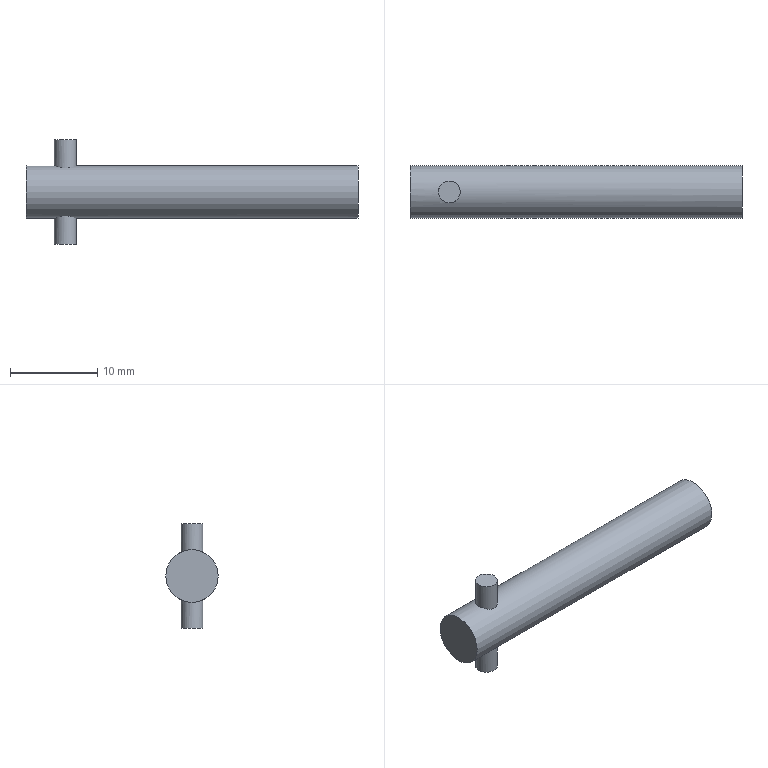Part | STEP file | 2-09.3 | 1 solid | 7 faces | box 38 x 6 x 12 mm | volume 1105 mm3 | plane 4 | cylinder 3 | commonest cylinder face diameters 2.5 x2 6 x1
STEP:
#1=CARTESIAN_POINT('',(0.,0.,0.));
#2=DIRECTION('',(0.,0.,1.));
#3=DIRECTION('',(1.,0.,0.));
#4=AXIS2_PLACEMENT_3D('',#1,#2,#3);
#5=CARTESIAN_POINT('',(0.,3.,0.));
#6=VERTEX_POINT('',#5);
#7=CARTESIAN_POINT('',(0.,0.,0.));
#8=DIRECTION('',(1.,0.,0.));
#9=DIRECTION('',(0.,1.,0.));
#10=AXIS2_PLACEMENT_3D('',#7,#8,#9);
#11=CIRCLE('',#10,3.);
#12=CARTESIAN_POINT('',(0.,-0.8038,0.));
#13=DIRECTION('',(1.,0.,0.));
#14=DIRECTION('',(0.,1.,0.));
#15=AXIS2_PLACEMENT_3D('',#12,#13,#14);
#16=PLANE('',#15);
#17=CARTESIAN_POINT('',(0.8038,0.));
#18=DIRECTION('',(1.,0.));
#19=AXIS2_PLACEMENT_2D('',#17,#18);
#20=CIRCLE('',#19,3.);
#21=(GEOMETRIC_REPRESENTATION_CONTEXT(2)PARAMETRIC_REPRESENTATION_CONTEXT()REPRESENTATION_CONTEXT('',''));
#22=DEFINITIONAL_REPRESENTATION('',(#20),#21);
#23=PCURVE('',#16,#22);
#24=CARTESIAN_POINT('',(0.,0.,0.));
#25=DIRECTION('',(1.,0.,0.));
#26=DIRECTION('',(0.,1.,0.));
#27=AXIS2_PLACEMENT_3D('',#24,#25,#26);
#28=CYLINDRICAL_SURFACE('',#27,3.);
#29=CARTESIAN_POINT('',(0.,0.));
#30=DIRECTION('',(1.,0.));
#31=VECTOR('',#30,1.);
#32=LINE('',#29,#31);
#33=(GEOMETRIC_REPRESENTATION_CONTEXT(2)PARAMETRIC_REPRESENTATION_CONTEXT()REPRESENTATION_CONTEXT('',''));
#34=DEFINITIONAL_REPRESENTATION('',(#32),#33);
#35=PCURVE('',#28,#34);
#36=SURFACE_CURVE('',#11,(#23,#35),.PCURVE_S1.);
#37=EDGE_CURVE('',#6,#6,#36,.T.);
#38=ORIENTED_EDGE('',*,*,#37,.T.);
#39=EDGE_LOOP('',(#38));
#40=FACE_BOUND('',#39,.F.);
#41=ADVANCED_FACE('',(#40),#16,.F.);
#42=CARTESIAN_POINT('',(38.,3.,0.));
#43=VERTEX_POINT('',#42);
#44=CARTESIAN_POINT('',(38.,0.,0.));
#45=DIRECTION('',(1.,0.,0.));
#46=DIRECTION('',(0.,1.,0.));
#47=AXIS2_PLACEMENT_3D('',#44,#45,#46);
#48=CIRCLE('',#47,3.);
#49=CARTESIAN_POINT('',(38.,-0.8038,0.));
#50=DIRECTION('',(1.,0.,0.));
#51=DIRECTION('',(0.,1.,0.));
#52=AXIS2_PLACEMENT_3D('',#49,#50,#51);
#53=PLANE('',#52);
#54=CARTESIAN_POINT('',(0.8038,0.));
#55=DIRECTION('',(1.,0.));
#56=AXIS2_PLACEMENT_2D('',#54,#55);
#57=CIRCLE('',#56,3.);
#58=(GEOMETRIC_REPRESENTATION_CONTEXT(2)PARAMETRIC_REPRESENTATION_CONTEXT()REPRESENTATION_CONTEXT('',''));
#59=DEFINITIONAL_REPRESENTATION('',(#57),#58);
#60=PCURVE('',#53,#59);
#61=CARTESIAN_POINT('',(0.,38.));
#62=DIRECTION('',(1.,0.));
#63=VECTOR('',#62,1.);
#64=LINE('',#61,#63);
#65=(GEOMETRIC_REPRESENTATION_CONTEXT(2)PARAMETRIC_REPRESENTATION_CONTEXT()REPRESENTATION_CONTEXT('',''));
#66=DEFINITIONAL_REPRESENTATION('',(#64),#65);
#67=PCURVE('',#28,#66);
#68=SURFACE_CURVE('',#48,(#60,#67),.PCURVE_S1.);
#69=EDGE_CURVE('',#43,#43,#68,.T.);
#70=ORIENTED_EDGE('',*,*,#69,.T.);
#71=EDGE_LOOP('',(#70));
#72=FACE_BOUND('',#71,.T.);
#73=ADVANCED_FACE('',(#72),#53,.T.);
#74=ORIENTED_EDGE('',*,*,#37,.T.);
#75=CARTESIAN_POINT('',(0.,3.,0.));
#76=DIRECTION('',(1.,0.,0.));
#77=VECTOR('',#76,1.);
#78=LINE('',#75,#77);
#79=CARTESIAN_POINT('',(6.283,0.));
#80=DIRECTION('',(0.,1.));
#81=VECTOR('',#80,1.);
#82=LINE('',#79,#81);
#83=(GEOMETRIC_REPRESENTATION_CONTEXT(2)PARAMETRIC_REPRESENTATION_CONTEXT()REPRESENTATION_CONTEXT('',''));
#84=DEFINITIONAL_REPRESENTATION('',(#82),#83);
#85=PCURVE('',#28,#84);
#86=CARTESIAN_POINT('',(0.,0.));
#87=DIRECTION('',(0.,1.));
#88=VECTOR('',#87,1.);
#89=LINE('',#86,#88);
#90=(GEOMETRIC_REPRESENTATION_CONTEXT(2)PARAMETRIC_REPRESENTATION_CONTEXT()REPRESENTATION_CONTEXT('',''));
#91=DEFINITIONAL_REPRESENTATION('',(#89),#90);
#92=PCURVE('',#28,#91);
#93=SEAM_CURVE('',#78,(#85,#92),.PCURVE_S1.);
#94=EDGE_CURVE('',#6,#43,#93,.T.);
#95=ORIENTED_EDGE('',*,*,#94,.T.);
#96=ORIENTED_EDGE('',*,*,#69,.F.);
#97=ORIENTED_EDGE('',*,*,#94,.F.);
#98=EDGE_LOOP('',(#74,#95,#96,#97));
#99=FACE_BOUND('',#98,.T.);
#100=CARTESIAN_POINT('',(3.25,0.,-3.));
#101=VERTEX_POINT('',#100);
#102=CARTESIAN_POINT('',(3.25,0.,-3.));
#103=CARTESIAN_POINT('',(3.25,0.187,-3.));
#104=CARTESIAN_POINT('',(3.376,0.7482,-2.948));
#105=CARTESIAN_POINT('',(3.851,1.128,-2.782));
#106=CARTESIAN_POINT('',(4.657,1.326,-2.694));
#107=CARTESIAN_POINT('',(5.12,1.178,-2.782));
#108=CARTESIAN_POINT('',(5.735,0.4976,-2.98));
#109=CARTESIAN_POINT('',(5.831,0.02602,-3.032));
#110=CARTESIAN_POINT('',(5.509,-0.9079,-2.903));
#111=CARTESIAN_POINT('',(5.038,-1.25,-2.727));
#112=CARTESIAN_POINT('',(3.853,-1.25,-2.727));
#113=CARTESIAN_POINT('',(3.315,-0.7572,-2.973));
#114=CARTESIAN_POINT('',(3.253,-0.08984,-2.999));
#115=CARTESIAN_POINT('',(3.251,-0.05135,-3.));
#116=CARTESIAN_POINT('',(3.25,-0.01284,-3.));
#117=CARTESIAN_POINT('',(3.25,0.,-3.));
#118=B_SPLINE_CURVE_WITH_KNOTS('',3,(#102,#103,#104,#105,#106,#107,#108,#109,#110,#111,#112,#113,#114,#115,#116,#117),.UNSPECIFIED.,.T.,.F.,(1,3,1,2,2,2,2,2,1,3,1),(-0.02386,0.,0.3333,1.,1.865,2.731,3.728,4.927,4.975,4.999,5.332),.UNSPECIFIED.);
#119=CARTESIAN_POINT('',(4.712,3.25));
#120=CARTESIAN_POINT('',(4.734,3.25));
#121=CARTESIAN_POINT('',(4.776,3.26));
#122=CARTESIAN_POINT('',(4.839,3.303));
#123=CARTESIAN_POINT('',(4.898,3.374));
#124=CARTESIAN_POINT('',(4.954,3.472));
#125=CARTESIAN_POINT('',(5.004,3.593));
#126=CARTESIAN_POINT('',(5.048,3.733));
#127=CARTESIAN_POINT('',(5.085,3.89));
#128=CARTESIAN_POINT('',(5.114,4.059));
#129=CARTESIAN_POINT('',(5.134,4.237));
#130=CARTESIAN_POINT('',(5.143,4.417));
#131=CARTESIAN_POINT('',(5.142,4.595));
#132=CARTESIAN_POINT('',(5.133,4.768));
#133=CARTESIAN_POINT('',(5.115,4.936));
#134=CARTESIAN_POINT('',(5.089,5.095));
#135=CARTESIAN_POINT('',(5.056,5.243));
#136=CARTESIAN_POINT('',(5.015,5.378));
#137=CARTESIAN_POINT('',(4.968,5.498));
#138=CARTESIAN_POINT('',(4.918,5.595));
#139=CARTESIAN_POINT('',(4.864,5.67));
#140=CARTESIAN_POINT('',(4.809,5.722));
#141=CARTESIAN_POINT('',(4.752,5.75));
#142=CARTESIAN_POINT('',(4.694,5.754));
#143=CARTESIAN_POINT('',(4.636,5.733));
#144=CARTESIAN_POINT('',(4.578,5.688));
#145=CARTESIAN_POINT('',(4.522,5.618));
#146=CARTESIAN_POINT('',(4.47,5.527));
#147=CARTESIAN_POINT('',(4.423,5.417));
#148=CARTESIAN_POINT('',(4.382,5.289));
#149=CARTESIAN_POINT('',(4.346,5.147));
#150=CARTESIAN_POINT('',(4.318,4.991));
#151=CARTESIAN_POINT('',(4.297,4.825));
#152=CARTESIAN_POINT('',(4.284,4.65));
#153=CARTESIAN_POINT('',(4.281,4.466));
#154=CARTESIAN_POINT('',(4.288,4.285));
#155=CARTESIAN_POINT('',(4.303,4.114));
#156=CARTESIAN_POINT('',(4.327,3.952));
#157=CARTESIAN_POINT('',(4.358,3.803));
#158=CARTESIAN_POINT('',(4.395,3.667));
#159=CARTESIAN_POINT('',(4.437,3.546));
#160=CARTESIAN_POINT('',(4.485,3.443));
#161=CARTESIAN_POINT('',(4.537,3.36));
#162=CARTESIAN_POINT('',(4.593,3.298));
#163=CARTESIAN_POINT('',(4.651,3.259));
#164=CARTESIAN_POINT('',(4.692,3.25));
#165=CARTESIAN_POINT('',(4.712,3.25));
#166=B_SPLINE_CURVE_WITH_KNOTS('',3,(#119,#120,#121,#122,#123,#124,#125,#126,#127,#128,#129,#130,#131,#132,#133,#134,#135,#136,#137,#138,#139,#140,#141,#142,#143,#144,#145,#146,#147,#148,#149,#150,#151,#152,#153,#154,#155,#156,#157,#158,#159,#160,#161,#162,#163,#164,#165),.UNSPECIFIED.,.T.,.F.,(4,1,1,1,1,1,1,1,1,1,1,1,1,1,1,1,1,1,1,1,1,1,1,1,1,1,1,1,1,1,1,1,1,1,1,1,1,1,1,1,1,1,1,1,4),(0.,0.1136,0.2272,0.3408,0.4544,0.568,0.6817,0.7953,0.9089,1.022,1.136,1.25,1.363,1.477,1.591,1.704,1.818,1.931,2.045,2.159,2.272,2.386,2.499,2.613,2.727,2.84,2.954,3.067,3.181,3.295,3.408,3.522,3.635,3.749,3.863,3.976,4.09,4.204,4.317,4.431,4.544,4.658,4.772,4.885,4.999),.QUASI_UNIFORM_KNOTS.);
#167=(GEOMETRIC_REPRESENTATION_CONTEXT(2)PARAMETRIC_REPRESENTATION_CONTEXT()REPRESENTATION_CONTEXT('',''));
#168=DEFINITIONAL_REPRESENTATION('',(#166),#167);
#169=PCURVE('',#28,#168);
#170=CARTESIAN_POINT('',(4.5,0.,-6.));
#171=DIRECTION('',(0.,0.,1.));
#172=DIRECTION('',(-1.,0.,0.));
#173=AXIS2_PLACEMENT_3D('',#170,#171,#172);
#174=CYLINDRICAL_SURFACE('',#173,1.25);
#175=CARTESIAN_POINT('',(6.283,3.));
#176=CARTESIAN_POINT('',(6.232,3.));
#177=CARTESIAN_POINT('',(6.13,3.004));
#178=CARTESIAN_POINT('',(5.978,3.021));
#179=CARTESIAN_POINT('',(5.826,3.048));
#180=CARTESIAN_POINT('',(5.674,3.084));
#181=CARTESIAN_POINT('',(5.523,3.124));
#182=CARTESIAN_POINT('',(5.372,3.166));
#183=CARTESIAN_POINT('',(5.221,3.205));
#184=CARTESIAN_POINT('',(5.072,3.239));
#185=CARTESIAN_POINT('',(4.924,3.262));
#186=CARTESIAN_POINT('',(4.779,3.272));
#187=CARTESIAN_POINT('',(4.637,3.27));
#188=CARTESIAN_POINT('',(4.497,3.257));
#189=CARTESIAN_POINT('',(4.358,3.236));
#190=CARTESIAN_POINT('',(4.219,3.207));
#191=CARTESIAN_POINT('',(4.078,3.173));
#192=CARTESIAN_POINT('',(3.937,3.136));
#193=CARTESIAN_POINT('',(3.792,3.096));
#194=CARTESIAN_POINT('',(3.651,3.063));
#195=CARTESIAN_POINT('',(3.512,3.036));
#196=CARTESIAN_POINT('',(3.374,3.016));
#197=CARTESIAN_POINT('',(3.236,3.004));
#198=CARTESIAN_POINT('',(3.098,3.001));
#199=CARTESIAN_POINT('',(2.958,3.008));
#200=CARTESIAN_POINT('',(2.815,3.025));
#201=CARTESIAN_POINT('',(2.671,3.053));
#202=CARTESIAN_POINT('',(2.53,3.086));
#203=CARTESIAN_POINT('',(2.39,3.123));
#204=CARTESIAN_POINT('',(2.251,3.161));
#205=CARTESIAN_POINT('',(2.113,3.197));
#206=CARTESIAN_POINT('',(1.973,3.229));
#207=CARTESIAN_POINT('',(1.833,3.254));
#208=CARTESIAN_POINT('',(1.69,3.27));
#209=CARTESIAN_POINT('',(1.543,3.275));
#210=CARTESIAN_POINT('',(1.399,3.266));
#211=CARTESIAN_POINT('',(1.258,3.247));
#212=CARTESIAN_POINT('',(1.119,3.219));
#213=CARTESIAN_POINT('',(0.9811,3.187));
#214=CARTESIAN_POINT('',(0.8438,3.15));
#215=CARTESIAN_POINT('',(0.7067,3.113));
#216=CARTESIAN_POINT('',(0.569,3.078));
#217=CARTESIAN_POINT('',(0.4304,3.046));
#218=CARTESIAN_POINT('',(0.2901,3.021));
#219=CARTESIAN_POINT('',(0.1469,3.004));
#220=CARTESIAN_POINT('',(0.04935,3.));
#221=CARTESIAN_POINT('',(0.,3.));
#222=B_SPLINE_CURVE_WITH_KNOTS('',3,(#175,#176,#177,#178,#179,#180,#181,#182,#183,#184,#185,#186,#187,#188,#189,#190,#191,#192,#193,#194,#195,#196,#197,#198,#199,#200,#201,#202,#203,#204,#205,#206,#207,#208,#209,#210,#211,#212,#213,#214,#215,#216,#217,#218,#219,#220,#221),.UNSPECIFIED.,.F.,.F.,(4,1,1,1,1,1,1,1,1,1,1,1,1,1,1,1,1,1,1,1,1,1,1,1,1,1,1,1,1,1,1,1,1,1,1,1,1,1,1,1,1,1,1,1,4),(0.,0.1136,0.2272,0.3408,0.4544,0.568,0.6817,0.7953,0.9089,1.022,1.136,1.25,1.363,1.477,1.591,1.704,1.818,1.931,2.045,2.159,2.272,2.386,2.499,2.613,2.727,2.84,2.954,3.067,3.181,3.295,3.408,3.522,3.635,3.749,3.863,3.976,4.09,4.204,4.317,4.431,4.544,4.658,4.772,4.885,4.999),.QUASI_UNIFORM_KNOTS.);
#223=(GEOMETRIC_REPRESENTATION_CONTEXT(2)PARAMETRIC_REPRESENTATION_CONTEXT()REPRESENTATION_CONTEXT('',''));
#224=DEFINITIONAL_REPRESENTATION('',(#222),#223);
#225=PCURVE('',#174,#224);
#226=SURFACE_CURVE('',#118,(#169,#225),.PCURVE_S1.);
#227=EDGE_CURVE('',#101,#101,#226,.T.);
#228=ORIENTED_EDGE('',*,*,#227,.F.);
#229=EDGE_LOOP('',(#228));
#230=FACE_BOUND('',#229,.T.);
#231=CARTESIAN_POINT('',(3.25,0.,3.));
#232=VERTEX_POINT('',#231);
#233=CARTESIAN_POINT('',(3.25,0.,3.));
#234=CARTESIAN_POINT('',(3.25,-0.188,3.));
#235=CARTESIAN_POINT('',(3.377,-0.7521,2.947));
#236=CARTESIAN_POINT('',(3.852,-1.13,2.781));
#237=CARTESIAN_POINT('',(4.617,-1.313,2.699));
#238=CARTESIAN_POINT('',(5.032,-1.203,2.763));
#239=CARTESIAN_POINT('',(5.678,-0.622,2.953));
#240=CARTESIAN_POINT('',(5.826,-0.1554,3.031));
#241=CARTESIAN_POINT('',(5.575,0.8598,2.929));
#242=CARTESIAN_POINT('',(5.074,1.25,2.727));
#243=CARTESIAN_POINT('',(3.846,1.25,2.727));
#244=CARTESIAN_POINT('',(3.309,0.7485,2.975));
#245=CARTESIAN_POINT('',(3.253,0.0826,2.999));
#246=CARTESIAN_POINT('',(3.251,0.04721,3.));
#247=CARTESIAN_POINT('',(3.25,0.0118,3.));
#248=CARTESIAN_POINT('',(3.25,0.,3.));
#249=B_SPLINE_CURVE_WITH_KNOTS('',3,(#233,#234,#235,#236,#237,#238,#239,#240,#241,#242,#243,#244,#245,#246,#247,#248),.UNSPECIFIED.,.T.,.F.,(1,3,1,2,2,2,2,2,1,3,1),(-0.02191,0.,0.3333,1.,1.762,2.619,3.67,4.868,4.912,4.934,5.267),.UNSPECIFIED.);
#250=CARTESIAN_POINT('',(1.571,3.25));
#251=CARTESIAN_POINT('',(1.592,3.25));
#252=CARTESIAN_POINT('',(1.634,3.26));
#253=CARTESIAN_POINT('',(1.696,3.302));
#254=CARTESIAN_POINT('',(1.755,3.371));
#255=CARTESIAN_POINT('',(1.81,3.467));
#256=CARTESIAN_POINT('',(1.86,3.585));
#257=CARTESIAN_POINT('',(1.904,3.723));
#258=CARTESIAN_POINT('',(1.942,3.878));
#259=CARTESIAN_POINT('',(1.971,4.045));
#260=CARTESIAN_POINT('',(1.991,4.223));
#261=CARTESIAN_POINT('',(2.001,4.404));
#262=CARTESIAN_POINT('',(2.001,4.583));
#263=CARTESIAN_POINT('',(1.992,4.758));
#264=CARTESIAN_POINT('',(1.975,4.927));
#265=CARTESIAN_POINT('',(1.949,5.088));
#266=CARTESIAN_POINT('',(1.916,5.238));
#267=CARTESIAN_POINT('',(1.874,5.377));
#268=CARTESIAN_POINT('',(1.828,5.495));
#269=CARTESIAN_POINT('',(1.778,5.592));
#270=CARTESIAN_POINT('',(1.725,5.668));
#271=CARTESIAN_POINT('',(1.669,5.72));
#272=CARTESIAN_POINT('',(1.611,5.749));
#273=CARTESIAN_POINT('',(1.552,5.753));
#274=CARTESIAN_POINT('',(1.492,5.732));
#275=CARTESIAN_POINT('',(1.432,5.684));
#276=CARTESIAN_POINT('',(1.376,5.612));
#277=CARTESIAN_POINT('',(1.325,5.52));
#278=CARTESIAN_POINT('',(1.278,5.408));
#279=CARTESIAN_POINT('',(1.237,5.279));
#280=CARTESIAN_POINT('',(1.202,5.135));
#281=CARTESIAN_POINT('',(1.174,4.978));
#282=CARTESIAN_POINT('',(1.154,4.81));
#283=CARTESIAN_POINT('',(1.142,4.634));
#284=CARTESIAN_POINT('',(1.14,4.45));
#285=CARTESIAN_POINT('',(1.147,4.271));
#286=CARTESIAN_POINT('',(1.163,4.101));
#287=CARTESIAN_POINT('',(1.187,3.941));
#288=CARTESIAN_POINT('',(1.218,3.793));
#289=CARTESIAN_POINT('',(1.255,3.659));
#290=CARTESIAN_POINT('',(1.298,3.54));
#291=CARTESIAN_POINT('',(1.346,3.439));
#292=CARTESIAN_POINT('',(1.397,3.358));
#293=CARTESIAN_POINT('',(1.452,3.297));
#294=CARTESIAN_POINT('',(1.51,3.259));
#295=CARTESIAN_POINT('',(1.55,3.25));
#296=CARTESIAN_POINT('',(1.571,3.25));
#297=B_SPLINE_CURVE_WITH_KNOTS('',3,(#250,#251,#252,#253,#254,#255,#256,#257,#258,#259,#260,#261,#262,#263,#264,#265,#266,#267,#268,#269,#270,#271,#272,#273,#274,#275,#276,#277,#278,#279,#280,#281,#282,#283,#284,#285,#286,#287,#288,#289,#290,#291,#292,#293,#294,#295,#296),.UNSPECIFIED.,.T.,.F.,(4,1,1,1,1,1,1,1,1,1,1,1,1,1,1,1,1,1,1,1,1,1,1,1,1,1,1,1,1,1,1,1,1,1,1,1,1,1,1,1,1,1,1,1,4),(0.,0.1121,0.2243,0.3364,0.4485,0.5607,0.6728,0.785,0.8971,1.009,1.121,1.234,1.346,1.458,1.57,1.682,1.794,1.906,2.018,2.131,2.243,2.355,2.467,2.579,2.691,2.803,2.916,3.028,3.14,3.252,3.364,3.476,3.588,3.701,3.813,3.925,4.037,4.149,4.261,4.373,4.485,4.598,4.71,4.822,4.934),.QUASI_UNIFORM_KNOTS.);
#298=(GEOMETRIC_REPRESENTATION_CONTEXT(2)PARAMETRIC_REPRESENTATION_CONTEXT()REPRESENTATION_CONTEXT('',''));
#299=DEFINITIONAL_REPRESENTATION('',(#297),#298);
#300=PCURVE('',#28,#299);
#301=CARTESIAN_POINT('',(4.5,0.,-6.));
#302=DIRECTION('',(0.,0.,1.));
#303=DIRECTION('',(-1.,0.,0.));
#304=AXIS2_PLACEMENT_3D('',#301,#302,#303);
#305=CYLINDRICAL_SURFACE('',#304,1.25);
#306=CARTESIAN_POINT('',(0.,9.));
#307=CARTESIAN_POINT('',(0.05061,9.));
#308=CARTESIAN_POINT('',(0.1518,8.996));
#309=CARTESIAN_POINT('',(0.3032,8.979));
#310=CARTESIAN_POINT('',(0.4537,8.953));
#311=CARTESIAN_POINT('',(0.6032,8.918));
#312=CARTESIAN_POINT('',(0.7527,8.878));
#313=CARTESIAN_POINT('',(0.902,8.836));
#314=CARTESIAN_POINT('',(1.051,8.797));
#315=CARTESIAN_POINT('',(1.2,8.764));
#316=CARTESIAN_POINT('',(1.348,8.739));
#317=CARTESIAN_POINT('',(1.494,8.728));
#318=CARTESIAN_POINT('',(1.637,8.729));
#319=CARTESIAN_POINT('',(1.778,8.741));
#320=CARTESIAN_POINT('',(1.918,8.762));
#321=CARTESIAN_POINT('',(2.059,8.79));
#322=CARTESIAN_POINT('',(2.2,8.824));
#323=CARTESIAN_POINT('',(2.345,8.864));
#324=CARTESIAN_POINT('',(2.487,8.901));
#325=CARTESIAN_POINT('',(2.627,8.935));
#326=CARTESIAN_POINT('',(2.767,8.962));
#327=CARTESIAN_POINT('',(2.906,8.984));
#328=CARTESIAN_POINT('',(3.046,8.997));
#329=CARTESIAN_POINT('',(3.187,9.));
#330=CARTESIAN_POINT('',(3.331,8.993));
#331=CARTESIAN_POINT('',(3.479,8.973));
#332=CARTESIAN_POINT('',(3.622,8.945));
#333=CARTESIAN_POINT('',(3.763,8.911));
#334=CARTESIAN_POINT('',(3.903,8.874));
#335=CARTESIAN_POINT('',(4.043,8.836));
#336=CARTESIAN_POINT('',(4.182,8.8));
#337=CARTESIAN_POINT('',(4.321,8.769));
#338=CARTESIAN_POINT('',(4.462,8.744));
#339=CARTESIAN_POINT('',(4.605,8.729));
#340=CARTESIAN_POINT('',(4.752,8.725));
#341=CARTESIAN_POINT('',(4.896,8.735));
#342=CARTESIAN_POINT('',(5.036,8.755));
#343=CARTESIAN_POINT('',(5.174,8.782));
#344=CARTESIAN_POINT('',(5.311,8.815));
#345=CARTESIAN_POINT('',(5.448,8.851));
#346=CARTESIAN_POINT('',(5.584,8.888));
#347=CARTESIAN_POINT('',(5.72,8.923));
#348=CARTESIAN_POINT('',(5.858,8.955));
#349=CARTESIAN_POINT('',(5.997,8.98));
#350=CARTESIAN_POINT('',(6.138,8.996));
#351=CARTESIAN_POINT('',(6.234,9.));
#352=CARTESIAN_POINT('',(6.283,9.));
#353=B_SPLINE_CURVE_WITH_KNOTS('',3,(#306,#307,#308,#309,#310,#311,#312,#313,#314,#315,#316,#317,#318,#319,#320,#321,#322,#323,#324,#325,#326,#327,#328,#329,#330,#331,#332,#333,#334,#335,#336,#337,#338,#339,#340,#341,#342,#343,#344,#345,#346,#347,#348,#349,#350,#351,#352),.UNSPECIFIED.,.F.,.F.,(4,1,1,1,1,1,1,1,1,1,1,1,1,1,1,1,1,1,1,1,1,1,1,1,1,1,1,1,1,1,1,1,1,1,1,1,1,1,1,1,1,1,1,1,4),(0.,0.1121,0.2243,0.3364,0.4485,0.5607,0.6728,0.785,0.8971,1.009,1.121,1.234,1.346,1.458,1.57,1.682,1.794,1.906,2.018,2.131,2.243,2.355,2.467,2.579,2.691,2.803,2.916,3.028,3.14,3.252,3.364,3.476,3.588,3.701,3.813,3.925,4.037,4.149,4.261,4.373,4.485,4.598,4.71,4.822,4.934),.QUASI_UNIFORM_KNOTS.);
#354=(GEOMETRIC_REPRESENTATION_CONTEXT(2)PARAMETRIC_REPRESENTATION_CONTEXT()REPRESENTATION_CONTEXT('',''));
#355=DEFINITIONAL_REPRESENTATION('',(#353),#354);
#356=PCURVE('',#305,#355);
#357=SURFACE_CURVE('',#249,(#300,#356),.PCURVE_S1.);
#358=EDGE_CURVE('',#232,#232,#357,.T.);
#359=ORIENTED_EDGE('',*,*,#358,.F.);
#360=EDGE_LOOP('',(#359));
#361=FACE_BOUND('',#360,.T.);
#362=ADVANCED_FACE('',(#99,#230,#361),#28,.T.);
#363=CARTESIAN_POINT('',(3.25,0.,-6.));
#364=VERTEX_POINT('',#363);
#365=CARTESIAN_POINT('',(4.5,0.,-6.));
#366=DIRECTION('',(0.,0.,1.));
#367=DIRECTION('',(-1.,0.,0.));
#368=AXIS2_PLACEMENT_3D('',#365,#366,#367);
#369=CIRCLE('',#368,1.25);
#370=CARTESIAN_POINT('',(0.,0.));
#371=DIRECTION('',(1.,0.));
#372=VECTOR('',#371,1.);
#373=LINE('',#370,#372);
#374=(GEOMETRIC_REPRESENTATION_CONTEXT(2)PARAMETRIC_REPRESENTATION_CONTEXT()REPRESENTATION_CONTEXT('',''));
#375=DEFINITIONAL_REPRESENTATION('',(#373),#374);
#376=PCURVE('',#174,#375);
#377=CARTESIAN_POINT('',(4.835,0.,-6.));
#378=DIRECTION('',(0.,0.,1.));
#379=DIRECTION('',(-1.,0.,0.));
#380=AXIS2_PLACEMENT_3D('',#377,#378,#379);
#381=PLANE('',#380);
#382=CARTESIAN_POINT('',(0.3349,0.));
#383=DIRECTION('',(1.,0.));
#384=AXIS2_PLACEMENT_2D('',#382,#383);
#385=CIRCLE('',#384,1.25);
#386=(GEOMETRIC_REPRESENTATION_CONTEXT(2)PARAMETRIC_REPRESENTATION_CONTEXT()REPRESENTATION_CONTEXT('',''));
#387=DEFINITIONAL_REPRESENTATION('',(#385),#386);
#388=PCURVE('',#381,#387);
#389=SURFACE_CURVE('',#369,(#376,#388),.PCURVE_S1.);
#390=EDGE_CURVE('',#364,#364,#389,.T.);
#391=ORIENTED_EDGE('',*,*,#390,.T.);
#392=CARTESIAN_POINT('',(3.25,0.,-6.));
#393=DIRECTION('',(0.,0.,1.));
#394=VECTOR('',#393,1.);
#395=LINE('',#392,#394);
#396=CARTESIAN_POINT('',(6.283,0.));
#397=DIRECTION('',(0.,1.));
#398=VECTOR('',#397,1.);
#399=LINE('',#396,#398);
#400=(GEOMETRIC_REPRESENTATION_CONTEXT(2)PARAMETRIC_REPRESENTATION_CONTEXT()REPRESENTATION_CONTEXT('',''));
#401=DEFINITIONAL_REPRESENTATION('',(#399),#400);
#402=PCURVE('',#174,#401);
#403=CARTESIAN_POINT('',(0.,0.));
#404=DIRECTION('',(0.,1.));
#405=VECTOR('',#404,1.);
#406=LINE('',#403,#405);
#407=(GEOMETRIC_REPRESENTATION_CONTEXT(2)PARAMETRIC_REPRESENTATION_CONTEXT()REPRESENTATION_CONTEXT('',''));
#408=DEFINITIONAL_REPRESENTATION('',(#406),#407);
#409=PCURVE('',#174,#408);
#410=SEAM_CURVE('',#395,(#402,#409),.PCURVE_S1.);
#411=EDGE_CURVE('',#364,#101,#410,.T.);
#412=ORIENTED_EDGE('',*,*,#411,.T.);
#413=ORIENTED_EDGE('',*,*,#227,.T.);
#414=ORIENTED_EDGE('',*,*,#411,.F.);
#415=EDGE_LOOP('',(#391,#412,#413,#414));
#416=FACE_BOUND('',#415,.T.);
#417=ADVANCED_FACE('',(#416),#174,.T.);
#418=CARTESIAN_POINT('',(3.25,0.,6.));
#419=VERTEX_POINT('',#418);
#420=CARTESIAN_POINT('',(4.5,0.,6.));
#421=DIRECTION('',(0.,0.,1.));
#422=DIRECTION('',(-1.,0.,0.));
#423=AXIS2_PLACEMENT_3D('',#420,#421,#422);
#424=CIRCLE('',#423,1.25);
#425=CARTESIAN_POINT('',(0.,12.));
#426=DIRECTION('',(1.,0.));
#427=VECTOR('',#426,1.);
#428=LINE('',#425,#427);
#429=(GEOMETRIC_REPRESENTATION_CONTEXT(2)PARAMETRIC_REPRESENTATION_CONTEXT()REPRESENTATION_CONTEXT('',''));
#430=DEFINITIONAL_REPRESENTATION('',(#428),#429);
#431=PCURVE('',#305,#430);
#432=CARTESIAN_POINT('',(4.835,0.,6.));
#433=DIRECTION('',(0.,0.,1.));
#434=DIRECTION('',(-1.,0.,0.));
#435=AXIS2_PLACEMENT_3D('',#432,#433,#434);
#436=PLANE('',#435);
#437=CARTESIAN_POINT('',(0.3349,0.));
#438=DIRECTION('',(1.,0.));
#439=AXIS2_PLACEMENT_2D('',#437,#438);
#440=CIRCLE('',#439,1.25);
#441=(GEOMETRIC_REPRESENTATION_CONTEXT(2)PARAMETRIC_REPRESENTATION_CONTEXT()REPRESENTATION_CONTEXT('',''));
#442=DEFINITIONAL_REPRESENTATION('',(#440),#441);
#443=PCURVE('',#436,#442);
#444=SURFACE_CURVE('',#424,(#431,#443),.PCURVE_S1.);
#445=EDGE_CURVE('',#419,#419,#444,.T.);
#446=ORIENTED_EDGE('',*,*,#445,.F.);
#447=CARTESIAN_POINT('',(3.25,0.,3.));
#448=DIRECTION('',(0.,0.,1.));
#449=VECTOR('',#448,1.);
#450=LINE('',#447,#449);
#451=CARTESIAN_POINT('',(0.,9.));
#452=DIRECTION('',(0.,1.));
#453=VECTOR('',#452,1.);
#454=LINE('',#451,#453);
#455=(GEOMETRIC_REPRESENTATION_CONTEXT(2)PARAMETRIC_REPRESENTATION_CONTEXT()REPRESENTATION_CONTEXT('',''));
#456=DEFINITIONAL_REPRESENTATION('',(#454),#455);
#457=PCURVE('',#305,#456);
#458=CARTESIAN_POINT('',(6.283,9.));
#459=DIRECTION('',(0.,1.));
#460=VECTOR('',#459,1.);
#461=LINE('',#458,#460);
#462=(GEOMETRIC_REPRESENTATION_CONTEXT(2)PARAMETRIC_REPRESENTATION_CONTEXT()REPRESENTATION_CONTEXT('',''));
#463=DEFINITIONAL_REPRESENTATION('',(#461),#462);
#464=PCURVE('',#305,#463);
#465=SEAM_CURVE('',#450,(#457,#464),.PCURVE_S1.);
#466=EDGE_CURVE('',#232,#419,#465,.T.);
#467=ORIENTED_EDGE('',*,*,#466,.F.);
#468=ORIENTED_EDGE('',*,*,#358,.T.);
#469=ORIENTED_EDGE('',*,*,#466,.T.);
#470=EDGE_LOOP('',(#446,#467,#468,#469));
#471=FACE_BOUND('',#470,.T.);
#472=ADVANCED_FACE('',(#471),#305,.T.);
#473=ORIENTED_EDGE('',*,*,#390,.T.);
#474=EDGE_LOOP('',(#473));
#475=FACE_BOUND('',#474,.F.);
#476=ADVANCED_FACE('',(#475),#381,.F.);
#477=ORIENTED_EDGE('',*,*,#445,.T.);
#478=EDGE_LOOP('',(#477));
#479=FACE_BOUND('',#478,.T.);
#480=ADVANCED_FACE('',(#479),#436,.T.);
#481=CLOSED_SHELL('',(#41,#73,#362,#417,#472,#476,#480));
#482=MANIFOLD_SOLID_BREP('',#481);
#483=(LENGTH_UNIT()NAMED_UNIT(*)SI_UNIT(.MILLI.,.METRE.));
#484=UNCERTAINTY_MEASURE_WITH_UNIT(LENGTH_MEASURE(0.001),#483,'','');
#485=(NAMED_UNIT(*)PLANE_ANGLE_UNIT()SI_UNIT($,.RADIAN.));
#486=(NAMED_UNIT(*)SI_UNIT($,.STERADIAN.)SOLID_ANGLE_UNIT());
#487=(GEOMETRIC_REPRESENTATION_CONTEXT(3)GLOBAL_UNCERTAINTY_ASSIGNED_CONTEXT((#484))GLOBAL_UNIT_ASSIGNED_CONTEXT((#483,#485,#486))REPRESENTATION_CONTEXT('',''));
#488=ADVANCED_BREP_SHAPE_REPRESENTATION('',(#4,#482),#487);